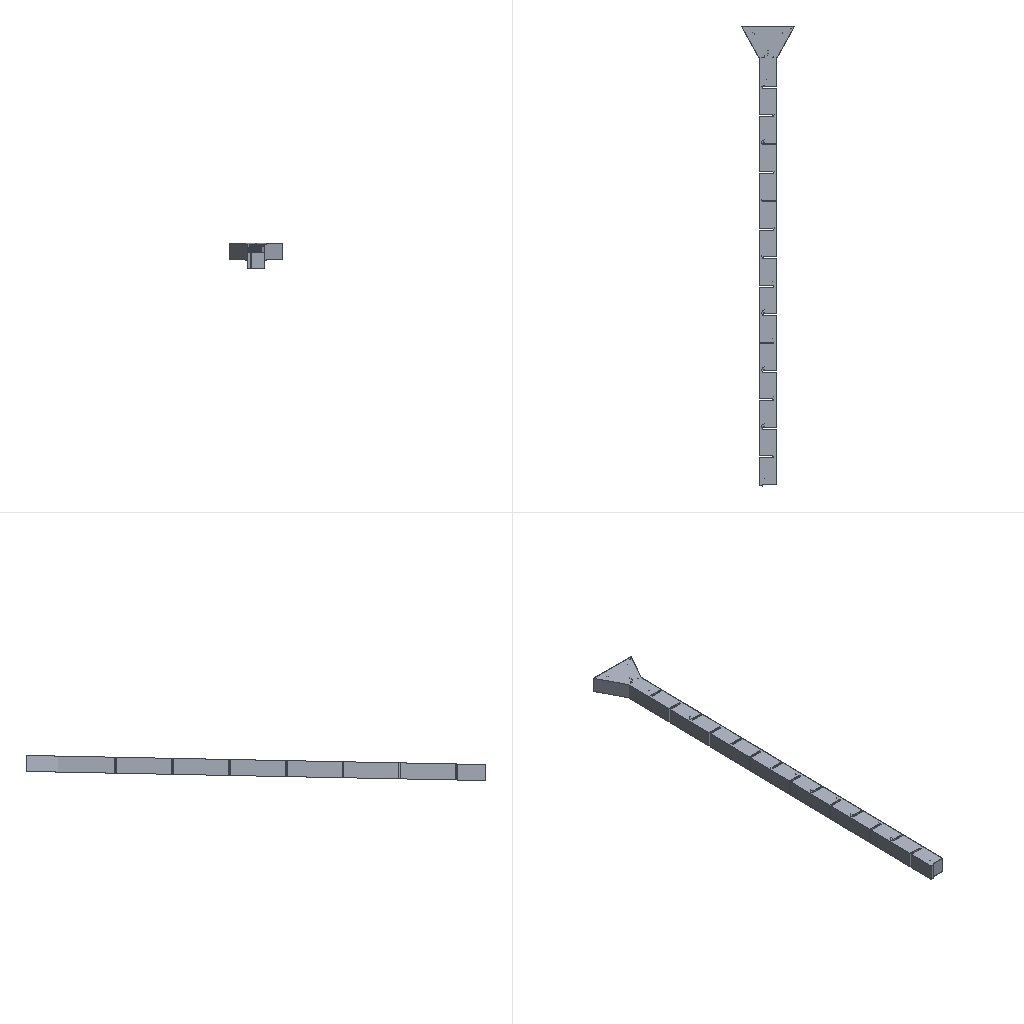Simulation study | ansys fluent
Set-up summary:
category,name,step,type,value,unit,region
solver,ansys_fluent,,Fluent 26.1.0
units,SI m-kg-s (Fluent internal),,stated,boundary values in the units shown in brackets; results in listed units
analysis,deck.cas,,cfd steady,"dimension=3D; solver=3d, dp, pbns, vof, rngke (3d, double precision, pressure-based, VOF, RNG k-epsilon); source_case=.cas"
model,Space,deck.cas,,3D
model,Time,deck.cas,,Steady
model,Viscous,deck.cas,,RNG k-epsilon turbulence model
model,Wall Treatment,deck.cas,,Standard Wall Functions
model,Heat Transfer,deck.cas,,Disabled
model,Multiphase,deck.cas,,Volume of Fluid
mesh,nodes,,,1639581
mesh,elements,,,1539648
mesh,faces,,,4717296
cell_zone,part_1 (mixture),deck.cas,fluid,material=water-liquid,,zone 3
cell_zone,part_1 (air),deck.cas,fluid,material=air,,zone 3
cell_zone,part_1 (water),deck.cas,fluid,material=water-liquid,,zone 3
material,water-liquid (fluid),,Density,998.2,kg/m^3
material,water-liquid (fluid),,Viscosity,0.001003,kg/(m s)
material,air (fluid),,Density,1.225,kg/m^3
material,air (fluid),,Viscosity,1.7894e-05,kg/(m s)
material,aluminum (solid),,Density,2719,kg/m^3
bc,out1 (mixture),deck.cas,pressure-outlet,Backflow Direction Specification Method=Normal to Boundary,,zone 7
bc,out1 (air),deck.cas,pressure-outlet,,,zone 7
bc,out1 (water),deck.cas,pressure-outlet,,,zone 7
bc,int (mixture),deck.cas,velocity-inlet,Velocity Magnitude [m/s]=0.8,,zone 6
bc,int (air),deck.cas,velocity-inlet,,,zone 6
bc,int (water),deck.cas,velocity-inlet,Volume Fraction=1,,zone 6
bc,wall-part_1 (mixture),deck.cas,wall,Wall Motion=Stationary Wall; Shear Boundary Condition=No Slip,,zone 1
bc,wall-part_1 (air),deck.cas,wall,,,zone 1
bc,wall-part_1 (water),deck.cas,wall,,,zone 1
bc,wall (mixture),deck.cas,wall,Wall Motion=Stationary Wall; Shear Boundary Condition=No Slip,,zone 8
bc,wall (air),deck.cas,wall,,,zone 8
bc,wall (water),deck.cas,wall,,,zone 8
bc,out (mixture),deck.cas,pressure-outlet,Backflow Direction Specification Method=Normal to Boundary,,zone 9
bc,out (air),deck.cas,pressure-outlet,,,zone 9
bc,out (water),deck.cas,pressure-outlet,,,zone 9
Results summary:
result,mass flow rate int,deck.cas,,8624.45,kg/s
result,mass flow rate out,deck.cas,,-227.932,kg/s
result,mass flow rate out1,deck.cas,,-8024.55,kg/s
result,mass flow rate wall,deck.cas,,-0,kg/s
result,mass flow rate wall-part_1,deck.cas,,-0,kg/s
result,mass flow rate Net,deck.cas,,371.967,kg/s
result,wall force total wall,deck.cas,,"(-1140.84, -46603.8, -1.00963e+06)",N
result,wall force pressure wall,deck.cas,,"(-1154.65, -46182.3, -1.00963e+06)",N
result,wall force viscous wall,deck.cas,,"(13.809, -421.516, 8.288)",N
result,wall force total wall-part_1,deck.cas,,"(1403.74, -48026.1, 33.255)",N
result,wall force pressure wall-part_1,deck.cas,,"(1401.42, -48009.5, 0)",N
result,wall force viscous wall-part_1,deck.cas,,"(2.321, -16.614, 33.255)",N
result,wall force total Net,deck.cas,,"(262.9, -94629.9, -1.00959e+06)",N
result,wall force pressure Net,deck.cas,,"(246.77, -94191.8, -1.00963e+06)",N
result,wall force viscous Net,deck.cas,,"(16.131, -438.13, 41.542)",N